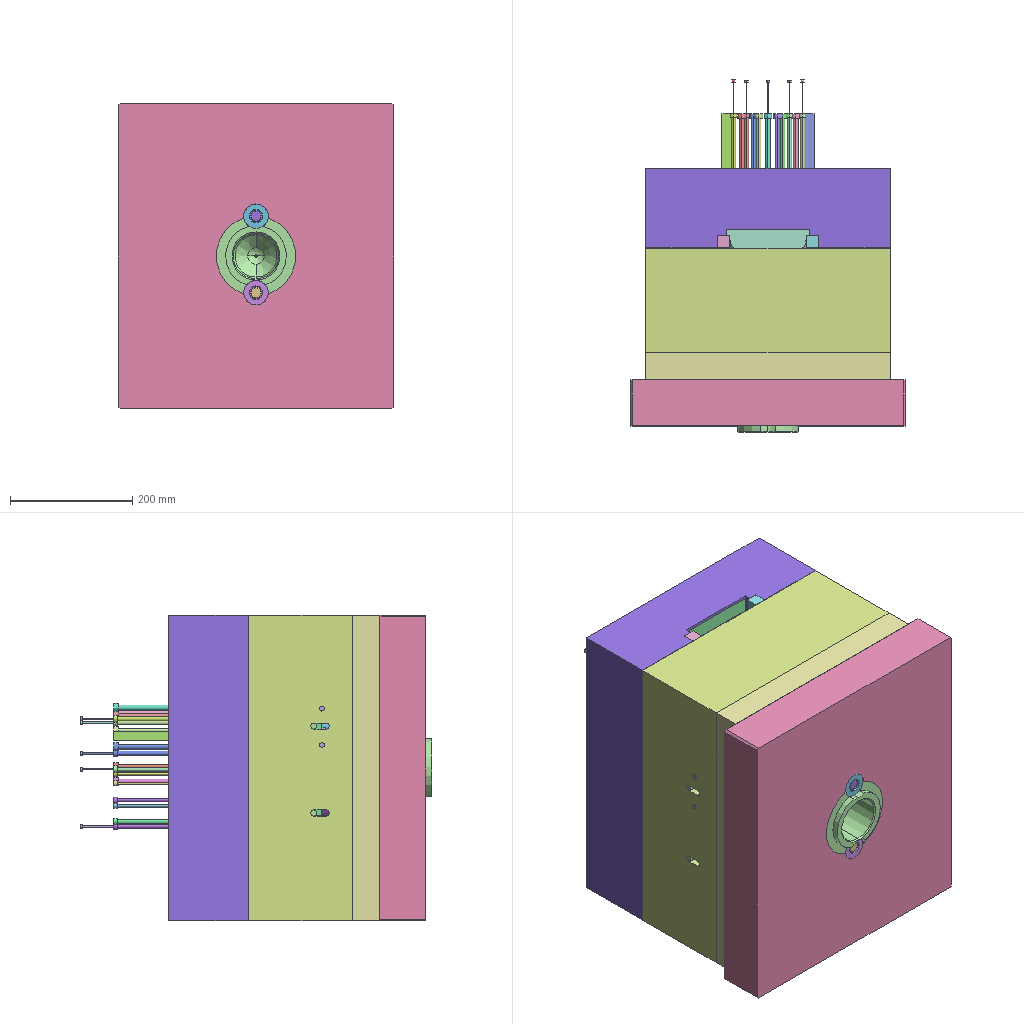Assembly | STEP file | 150 different items | 150 placed | box 450 x 576 x 500 mm
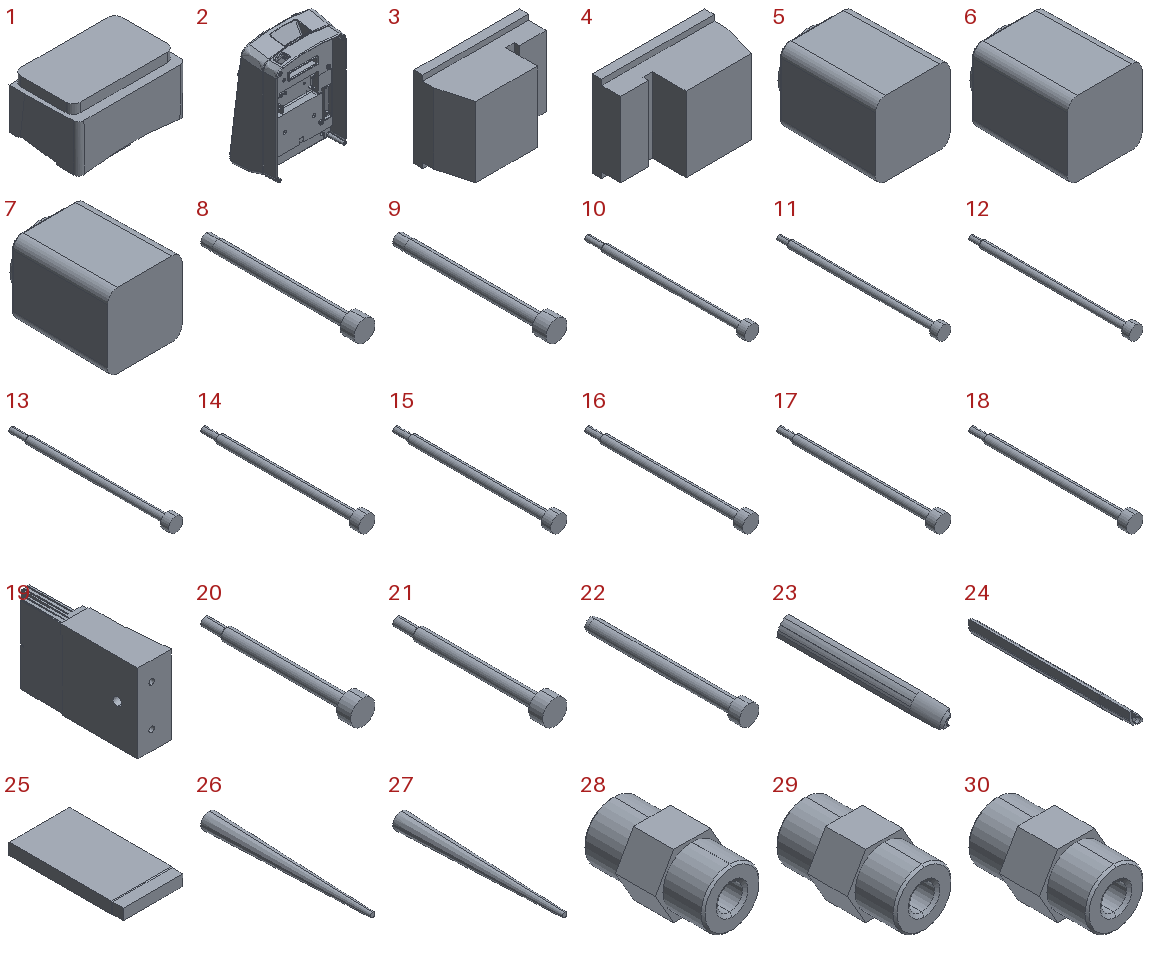Parts list (item | name | quantity | size | volume):
1 | (subassembly) | x1 | 119.805 x 74.045 x 84.64 mm | 483562 mm3
2 | 6022D002A | x1 | 145.669 x 91.672 x 216.186 mm | 218692 mm3
3 | (subassembly) | x1 | 60 x 30 x 46 mm | 59329 mm3
4 | (subassembly) | x1 | 60 x 30 x 46 mm | 59329 mm3
5 | (subassembly) | x1 | 11.23 x 15.729 x 11.23 mm | 1839 mm3
6 | (subassembly) | x1 | 11.23 x 15.729 x 11.23 mm | 1839 mm3
7 | (subassembly) | x1 | 11.23 x 15.729 x 11.23 mm | 1839 mm3
8 | (subassembly) | x1 | 9 x 68.14 x 9 mm | 1598 mm3
9 | (subassembly) | x1 | 9 x 68.14 x 9 mm | 1598 mm3
10 | (subassembly) | x1 | 7 x 79.697 x 7 mm | 843.527 mm3
11 | (subassembly) | x1 | 7 x 84.723 x 7 mm | 901.172 mm3
12 | (subassembly) | x1 | 7 x 84.723 x 7 mm | 901.172 mm3
13 | (subassembly) | x1 | 7 x 79.697 x 7 mm | 843.527 mm3
14 | (subassembly) | x1 | 7 x 69.447 x 7 mm | 750.263 mm3
15 | (subassembly) | x1 | 7 x 69.447 x 7 mm | 750.263 mm3
16 | (subassembly) | x1 | 7 x 69.447 x 7 mm | 750.263 mm3
17 | (subassembly) | x1 | 7 x 69.447 x 7 mm | 750.263 mm3
18 | (subassembly) | x1 | 7 x 69.447 x 7 mm | 750.263 mm3
19 | (subassembly) | x1 | 24.206 x 92.813 x 57.276 mm | 94075 mm3
20 | (subassembly) | x1 | 7 x 45.025 x 7 mm | 517.748 mm3
21 | (subassembly) | x1 | 7 x 45.025 x 7 mm | 517.748 mm3
22 | (subassembly) | x1 | 10 x 80.703 x 10 mm | 2941 mm3
23 | (subassembly) | x1 | 8.776 x 127.988 x 11.283 mm | 8417 mm3
24 | (subassembly) | x1 | 8.776 x 127.988 x 11.283 mm | 8418 mm3
25 | (subassembly) | x1 | 56.208 x 106.38 x 10.782 mm | 63955 mm3
26 | (subassembly) | x1 | 12.021 x 121.757 x 12.021 mm | 6349 mm3
27 | (subassembly) | x1 | 12.021 x 121.757 x 12.021 mm | 6349 mm3
28 | 6022D044 | x1 | 7.332 x 12 x 6.35 mm | 290.823 mm3
29 | 6022D044-1 | x1 | 7.332 x 12 x 6.35 mm | 290.823 mm3
30 | 6022D044-2 | x1 | 7.332 x 12 x 6.35 mm | 290.823 mm3
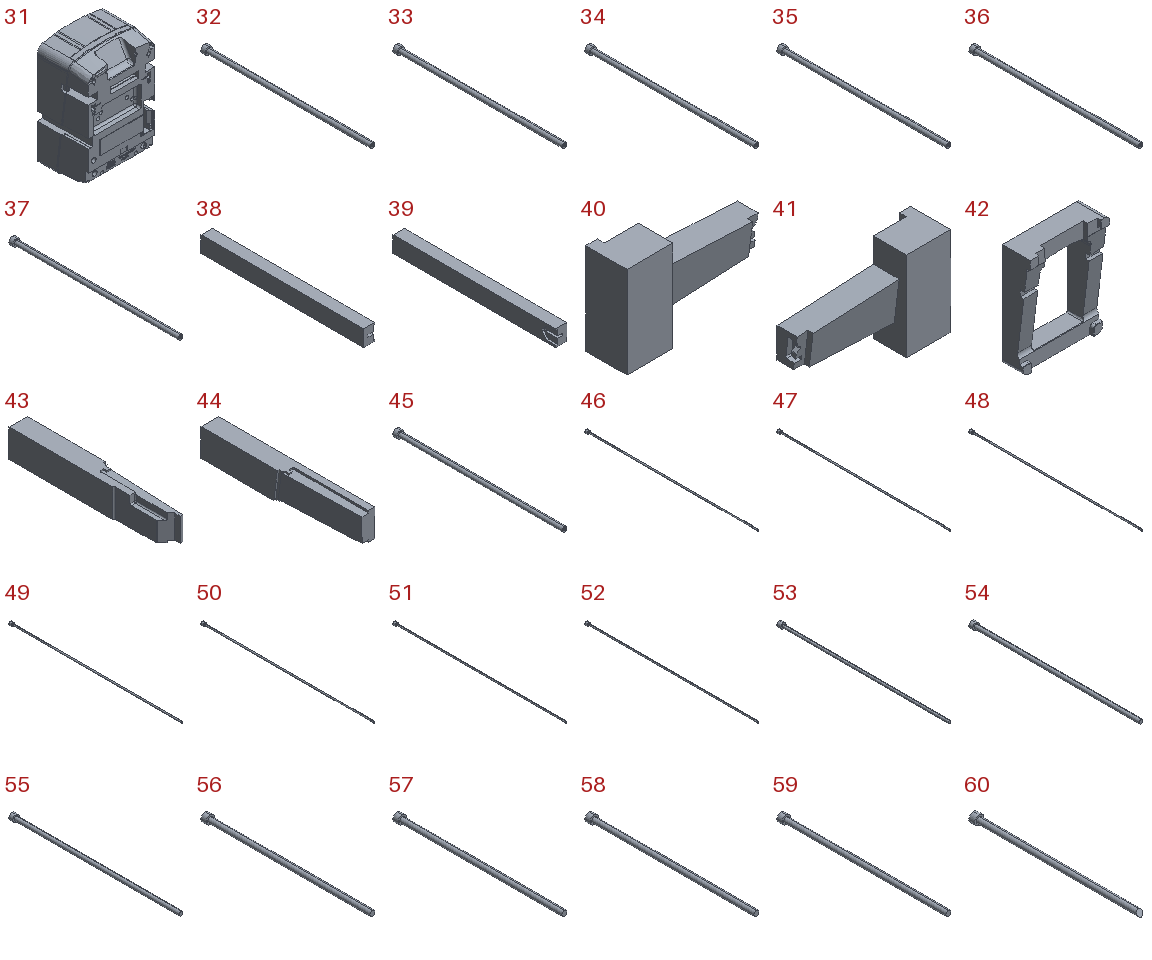31 | (subassembly) | x1 | 143.116 x 106.38 x 213.742 mm | 2647333 mm3
32 | (subassembly) | x1 | 11 x 244.986 x 11 mm | 8542 mm3
33 | (subassembly) | x1 | 11 x 244.986 x 11 mm | 8542 mm3
34 | (subassembly) | x1 | 11 x 244.986 x 11 mm | 8542 mm3
35 | (subassembly) | x1 | 11 x 244.986 x 11 mm | 8542 mm3
36 | (subassembly) | x1 | 11 x 243.265 x 11 mm | 8491 mm3
37 | (subassembly) | x1 | 11 x 254.534 x 11 mm | 8863 mm3
38 | (subassembly) | x1 | 7 x 102.36 x 10.193 mm | 7206 mm3
39 | (subassembly) | x1 | 7 x 102.36 x 10.193 mm | 7206 mm3
40 | (subassembly) | x1 | 63.268 x 18 x 40 mm | 19584 mm3
41 | (subassembly) | x1 | 63.268 x 18 x 40 mm | 19584 mm3
42 | (subassembly) | x1 | 220 x 78 x 290 mm | 1840139 mm3
43 | (subassembly) | x1 | 11.534 x 102.36 x 18.001 mm | 17054 mm3
44 | (subassembly) | x1 | 11.534 x 102.36 x 18.001 mm | 18637 mm3
45 | (subassembly) | x1 | 11 x 254.534 x 11 mm | 8863 mm3
46 | (subassembly) | x1 | 6 x 312.335 x 6 mm | 1622 mm3
47 | (subassembly) | x1 | 6 x 312.335 x 6 mm | 1622 mm3
48 | (subassembly) | x1 | 6 x 304.798 x 6 mm | 1589 mm3
49 | (subassembly) | x1 | 6 x 306.305 x 6 mm | 1597 mm3
50 | (subassembly) | x1 | 6 x 304.798 x 6 mm | 1589 mm3
51 | (subassembly) | x1 | 6 x 317.863 x 6 mm | 1651 mm3
52 | (subassembly) | x1 | 6 x 317.863 x 6 mm | 1651 mm3
53 | (subassembly) | x1 | 8 x 262.36 x 8 mm | 3523 mm3
54 | (subassembly) | x1 | 10 x 262.36 x 10 mm | 7720 mm3
55 | (subassembly) | x1 | 10 x 262.36 x 10 mm | 7720 mm3
56 | (subassembly) | x1 | 13 x 262.36 x 13 mm | 13847 mm3
57 | (subassembly) | x1 | 13 x 262.36 x 13 mm | 13847 mm3
58 | (subassembly) | x1 | 13 x 262.36 x 13 mm | 13847 mm3
59 | (subassembly) | x1 | 13 x 262.36 x 13 mm | 13847 mm3
60 | (subassembly) | x1 | 13 x 237.193 x 13 mm | 12467 mm3
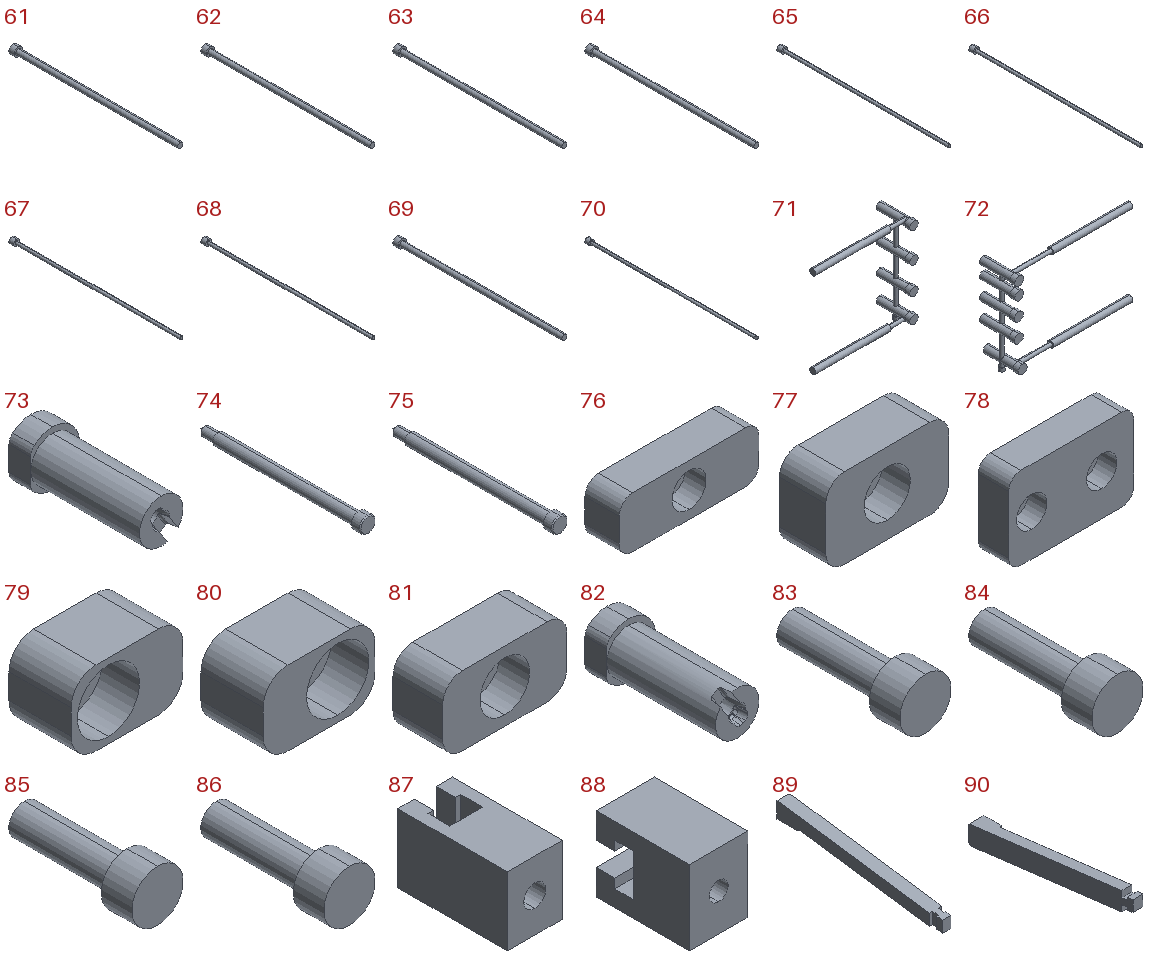61 | (subassembly) | x1 | 13 x 257.335 x 13 mm | 13595 mm3
62 | (subassembly) | x1 | 13 x 262.36 x 13 mm | 13847 mm3
63 | (subassembly) | x1 | 13 x 262.36 x 13 mm | 13847 mm3
64 | (subassembly) | x1 | 13 x 262.36 x 13 mm | 13847 mm3
65 | (subassembly) | x1 | 8 x 229.999 x 8 mm | 3116 mm3
66 | (subassembly) | x1 | 8 x 229.999 x 8 mm | 3116 mm3
67 | (subassembly) | x1 | 8 x 223.165 x 8 mm | 3031 mm3
68 | (subassembly) | x1 | 8 x 223.165 x 8 mm | 3031 mm3
69 | (subassembly) | x1 | 13 x 262.36 x 13 mm | 13847 mm3
70 | (subassembly) | x1 | 8 x 258.534 x 8 mm | 3450 mm3
71 | (subassembly) | x1 | 162 x 60 x 158.144 mm | 51671 mm3
72 | (subassembly) | x1 | 195 x 60 x 147.144 mm | 59737 mm3
73 | (subassembly) | x1 | 22.5 x 60 x 25 mm | 17728 mm3
74 | (subassembly) | x1 | 18 x 190 x 18 mm | 25064 mm3
75 | (subassembly) | x1 | 18 x 190 x 18 mm | 25064 mm3
76 | (subassembly) | x1 | 41 x 10 x 15 mm | 5428 mm3
77 | (subassembly) | x1 | 26.5 x 10 x 17.347 mm | 3875 mm3
78 | (subassembly) | x1 | 41 x 10 x 27 mm | 9764 mm3
79 | (subassembly) | x1 | 18 x 10 x 12 mm | 1438 mm3
80 | (subassembly) | x1 | 18 x 10 x 12 mm | 1438 mm3
81 | (subassembly) | x1 | 25.075 x 10 x 14 mm | 2789 mm3
82 | (subassembly) | x1 | 22.5 x 60 x 25 mm | 17728 mm3
83 | (subassembly) | x1 | 10 x 26 x 10 mm | 1037 mm3
84 | (subassembly) | x1 | 10 x 26 x 10 mm | 1037 mm3
85 | (subassembly) | x1 | 10 x 26 x 10 mm | 1037 mm3
86 | (subassembly) | x1 | 10 x 26 x 10 mm | 1037 mm3
87 | (subassembly) | x1 | 10 x 20 x 12.5 mm | 1868 mm3
88 | (subassembly) | x1 | 12.5 x 20 x 16 mm | 3149 mm3
89 | (subassembly) | x1 | 9 x 116.693 x 24.479 mm | 8518 mm3
90 | (subassembly) | x1 | 24.479 x 116.693 x 15 mm | 14289 mm3
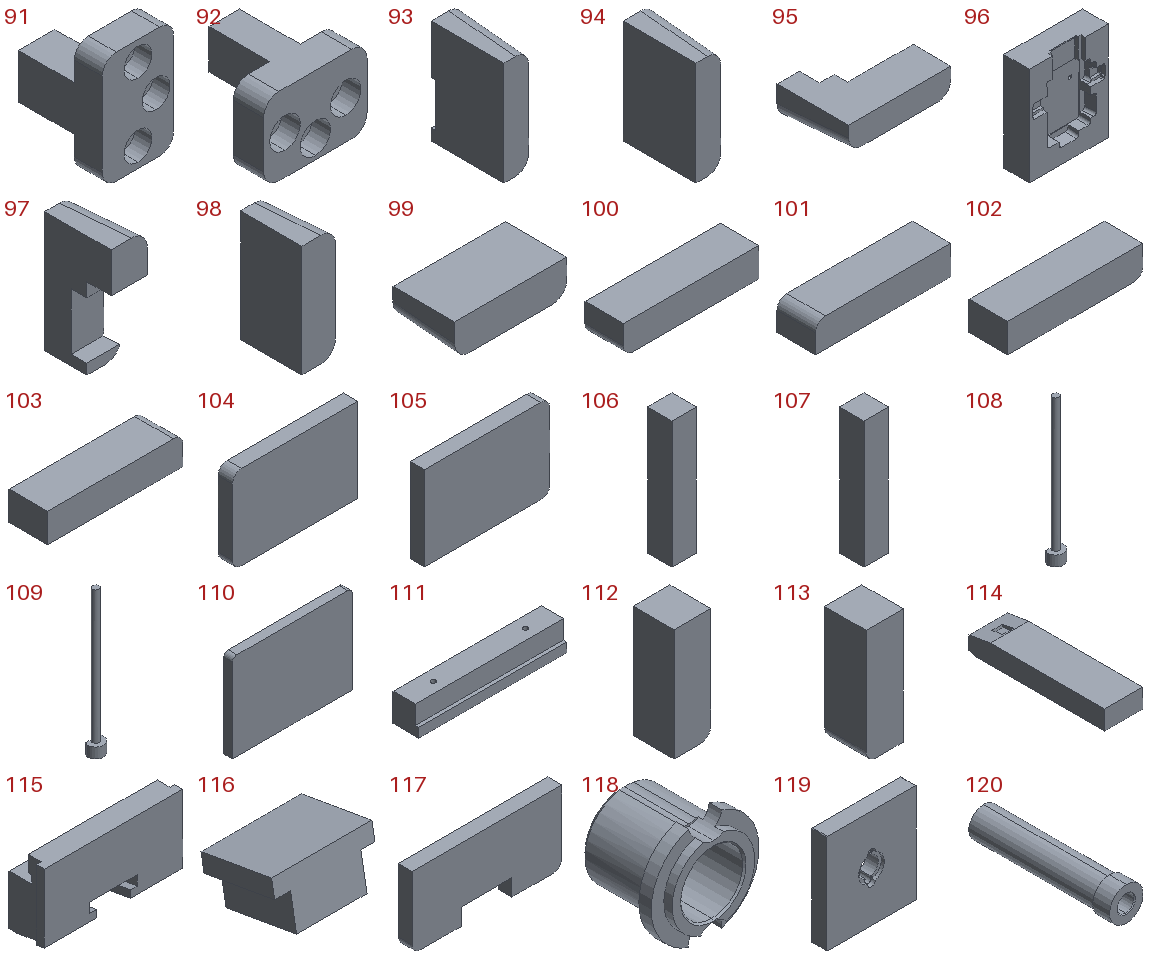91 | (subassembly) | x1 | 25.5 x 30 x 40 mm | 12392 mm3
92 | (subassembly) | x1 | 34 x 30 x 25.5 mm | 9302 mm3
93 | (subassembly) | x1 | 30 x 70 x 100 mm | 177836 mm3
94 | (subassembly) | x1 | 30 x 70 x 100 mm | 183468 mm3
95 | (subassembly) | x1 | 100 x 70 x 30 mm | 115912 mm3
96 | (subassembly) | x1 | 400 x 130 x 500 mm | 20837897 mm3
97 | (subassembly) | x1 | 30 x 55 x 100 mm | 92612 mm3
98 | (subassembly) | x1 | 30 x 55 x 100 mm | 147763 mm3
99 | (subassembly) | x1 | 100 x 55 x 30 mm | 147763 mm3
100 | (subassembly) | x1 | 70 x 20 x 15 mm | 20893 mm3
101 | (subassembly) | x1 | 70 x 20 x 15 mm | 20893 mm3
102 | (subassembly) | x1 | 70 x 20 x 15 mm | 20893 mm3
103 | (subassembly) | x1 | 70 x 20 x 15 mm | 20893 mm3
104 | (subassembly) | x1 | 70 x 8 x 47 mm | 26234 mm3
105 | (subassembly) | x1 | 70 x 8 x 47 mm | 26234 mm3
106 | (subassembly) | x1 | 20 x 20 x 105 mm | 42000 mm3
107 | (subassembly) | x1 | 20 x 20 x 105 mm | 42000 mm3
108 | (subassembly) | x1 | 6 x 4.256 x 55.458 mm | 340.576 mm3
109 | (subassembly) | x1 | 6 x 4.256 x 55.458 mm | 340.576 mm3
110 | (subassembly) | x1 | 136 x 10 x 100 mm | 135893 mm3
111 | (subassembly) | x1 | 80 x 14 x 15 mm | 14919 mm3
112 | (subassembly) | x1 | 18 x 20 x 55 mm | 19693 mm3
113 | (subassembly) | x1 | 18 x 20 x 56 mm | 20053 mm3
114 | (subassembly) | x1 | 70 x 250 x 35 mm | 599290 mm3
115 | (subassembly) | x1 | 86 x 25 x 46 mm | 68378 mm3
116 | (subassembly) | x1 | 28.5 x 22.681 x 18.312 mm | 6982 mm3
117 | (subassembly) | x1 | 87 x 8 x 41.949 mm | 26801 mm3
118 | (subassembly) | x1 | 130 x 132.5 x 123.637 mm | 522073 mm3
119 | (subassembly) | x1 | 450 x 75 x 500 mm | 16040639 mm3
120 | (subassembly) | x1 | 40 x 170 x 40 mm | 118148 mm3
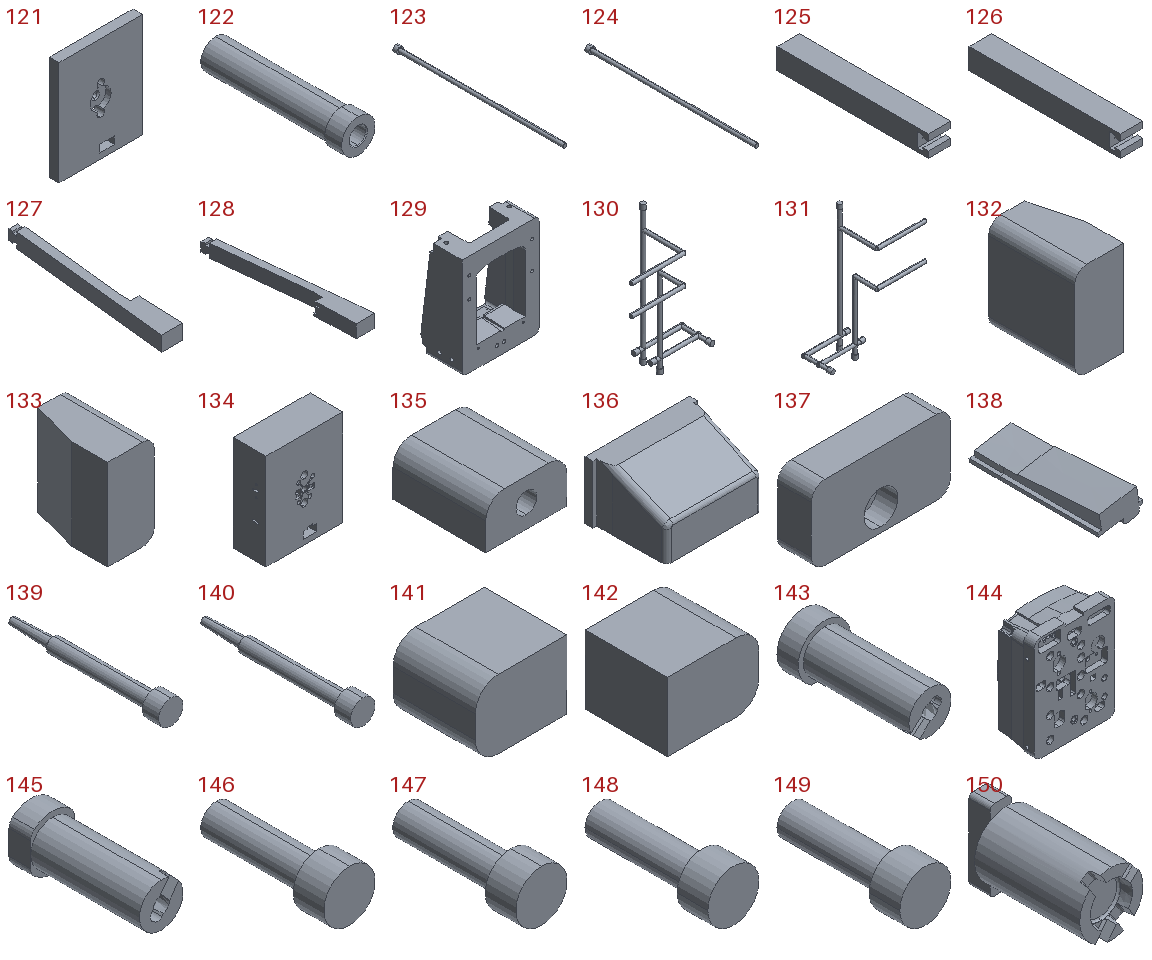121 | (subassembly) | x1 | 400 x 45 x 500 mm | 8595426 mm3
122 | (subassembly) | x1 | 40 x 170 x 40 mm | 118148 mm3
123 | (subassembly) | x1 | 10 x 257.335 x 10 mm | 7578 mm3
124 | (subassembly) | x1 | 10 x 257.335 x 10 mm | 7578 mm3
125 | (subassembly) | x1 | 16 x 108 x 15 mm | 24896 mm3
126 | (subassembly) | x1 | 16 x 108 x 15 mm | 24896 mm3
127 | (subassembly) | x1 | 24.981 x 162.36 x 14 mm | 24299 mm3
128 | (subassembly) | x1 | 24.981 x 162.36 x 14 mm | 24299 mm3
129 | (subassembly) | x1 | 220 x 118.069 x 290 mm | 3396178 mm3
130 | (subassembly) | x1 | 195 x 94 x 290 mm | 55392 mm3
131 | (subassembly) | x1 | 195 x 94 x 290 mm | 54387 mm3
132 | (subassembly) | x1 | 20 x 35.5 x 39 mm | 25224 mm3
133 | (subassembly) | x1 | 20 x 35.5 x 39 mm | 25224 mm3
134 | (subassembly) | x1 | 400 x 170 x 500 mm | 24400760 mm3
135 | (subassembly) | x1 | 35 x 40 x 20 mm | 23544 mm3
136 | (subassembly) | x1 | 135 x 99.045 x 75 mm | 726805 mm3
137 | (subassembly) | x1 | 41 x 10 x 22 mm | 8298 mm3
138 | (subassembly) | x1 | 21.719 x 62.11 x 12.971 mm | 7839 mm3
139 | (subassembly) | x1 | 6 x 38.743 x 6 mm | 385.655 mm3
140 | (subassembly) | x1 | 6 x 38.743 x 6 mm | 385.655 mm3
141 | (subassembly) | x1 | 20 x 18 x 15 mm | 5207 mm3
142 | (subassembly) | x1 | 20 x 18 x 15 mm | 5207 mm3
143 | (subassembly) | x1 | 25 x 60 x 23.412 mm | 17876 mm3
144 | (subassembly) | x1 | 150 x 88.701 x 195 mm | 1700421 mm3
145 | (subassembly) | x1 | 20 x 60 x 25 mm | 17460 mm3
146 | (subassembly) | x1 | 10 x 26 x 10 mm | 1037 mm3
147 | (subassembly) | x1 | 10 x 26 x 10 mm | 1037 mm3
148 | (subassembly) | x1 | 10 x 26 x 10 mm | 1037 mm3
149 | (subassembly) | x1 | 10 x 26 x 10 mm | 1037 mm3
150 | (subassembly) | x1 | 30 x 60 x 38 mm | 36750 mm3
Placements (level | parent | child | x y z in mm | rotation matrix by rows):
1 | subassembly 2 | subassembly 3 | -0.0 -0.0 -0.0 | 1 0 0 0 1 0 0 0 1
1 | subassembly 2 | 6022D002A | -0.0 -0.0 -0.0 | 1 0 0 0 1 0 0 0 1
1 | subassembly 2 | subassembly 4 | -0.0 -0.0 -0.0 | 1 0 0 0 1 0 0 0 1
1 | subassembly 2 | subassembly 5 | -0.0 -0.0 -0.0 | 1 0 0 0 1 0 0 0 1
1 | subassembly 2 | subassembly 6 | -0.0 -0.0 -0.0 | 1 0 0 0 1 0 0 0 1
1 | subassembly 2 | subassembly 7 | -0.0 -0.0 -0.0 | 1 0 0 0 1 0 0 0 1
1 | subassembly 2 | subassembly 8 | -0.0 -0.0 -0.0 | 1 0 0 0 1 0 0 0 1
1 | subassembly 2 | subassembly 9 | -0.0 -0.0 -0.0 | 1 0 0 0 1 0 0 0 1
1 | subassembly 2 | subassembly 10 | -0.0 -0.0 -0.0 | 1 0 0 0 1 0 0 0 1
1 | subassembly 2 | subassembly 11 | -0.0 -0.0 -0.0 | 1 0 0 0 1 0 0 0 1
1 | subassembly 2 | subassembly 12 | -0.0 -0.0 -0.0 | 1 0 0 0 1 0 0 0 1
1 | subassembly 2 | subassembly 13 | -0.0 -0.0 -0.0 | 1 0 0 0 1 0 0 0 1
1 | subassembly 2 | subassembly 14 | -0.0 -0.0 -0.0 | 1 0 0 0 1 0 0 0 1
1 | subassembly 2 | subassembly 15 | -0.0 -0.0 -0.0 | 1 0 0 0 1 0 0 0 1
1 | subassembly 2 | subassembly 16 | -0.0 -0.0 -0.0 | 1 0 0 0 1 0 0 0 1
1 | subassembly 2 | subassembly 17 | -0.0 -0.0 -0.0 | 1 0 0 0 1 0 0 0 1
1 | subassembly 2 | subassembly 18 | -0.0 -0.0 -0.0 | 1 0 0 0 1 0 0 0 1
1 | subassembly 2 | subassembly 19 | -0.0 -0.0 -0.0 | 1 0 0 0 1 0 0 0 1
1 | subassembly 2 | subassembly 20 | -0.0 -0.0 -0.0 | 1 0 0 0 1 0 0 0 1
1 | subassembly 2 | subassembly 21 | -0.0 -0.0 -0.0 | 1 0 0 0 1 0 0 0 1
1 | subassembly 2 | subassembly 22 | -0.0 -0.0 -0.0 | 1 0 0 0 1 0 0 0 1
1 | subassembly 2 | subassembly 23 | -0.0 -0.0 -0.0 | 1 0 0 0 1 0 0 0 1
1 | subassembly 2 | subassembly 24 | -0.0 -0.0 -0.0 | 1 0 0 0 1 0 0 0 1
1 | subassembly 2 | subassembly 25 | -0.0 -0.0 -0.0 | 1 0 0 0 1 0 0 0 1
1 | subassembly 2 | subassembly 26 | -0.0 -0.0 -0.0 | 1 0 0 0 1 0 0 0 1
1 | subassembly 2 | subassembly 27 | -0.0 -0.0 -0.0 | 1 0 0 0 1 0 0 0 1
1 | subassembly 2 | subassembly 28 | -0.0 -0.0 -0.0 | 1 0 0 0 1 0 0 0 1
1 | subassembly 2 | 6022D044 | -0.0 -0.0 -0.0 | 1 0 0 0 1 0 0 0 1
1 | subassembly 2 | 6022D044-1 | -0.0 -0.0 -0.0 | 1 0 0 0 1 0 0 0 1
1 | subassembly 2 | 6022D044-2 | -0.0 -0.0 -0.0 | 1 0 0 0 1 0 0 0 1
1 | subassembly 2 | subassembly 29 | -0.0 -0.0 -0.0 | 1 0 0 0 1 0 0 0 1
1 | subassembly 2 | subassembly 30 | -0.0 -0.0 -0.0 | 1 0 0 0 1 0 0 0 1
1 | subassembly 2 | subassembly 31 | -0.0 -0.0 -0.0 | 1 0 0 0 1 0 0 0 1
1 | subassembly 2 | subassembly 32 | -0.0 -0.0 -0.0 | 1 0 0 0 1 0 0 0 1
1 | subassembly 2 | subassembly 33 | -0.0 -0.0 -0.0 | 1 0 0 0 1 0 0 0 1
1 | subassembly 2 | subassembly 34 | -0.0 -0.0 -0.0 | 1 0 0 0 1 0 0 0 1
1 | subassembly 2 | subassembly 35 | -0.0 -0.0 -0.0 | 1 0 0 0 1 0 0 0 1
1 | subassembly 2 | subassembly 36 | -0.0 -0.0 -0.0 | 1 0 0 0 1 0 0 0 1
1 | subassembly 2 | subassembly 37 | -0.0 -0.0 -0.0 | 1 0 0 0 1 0 0 0 1
1 | subassembly 2 | subassembly 38 | -0.0 -0.0 -0.0 | 1 0 0 0 1 0 0 0 1
1 | subassembly 2 | subassembly 39 | -0.0 -0.0 -0.0 | 1 0 0 0 1 0 0 0 1
1 | subassembly 2 | subassembly 40 | -0.0 -0.0 -0.0 | 1 0 0 0 1 0 0 0 1
1 | subassembly 2 | subassembly 41 | -0.0 -0.0 -0.0 | 1 0 0 0 1 0 0 0 1
1 | subassembly 2 | subassembly 42 | -0.0 -0.0 -0.0 | 1 0 0 0 1 0 0 0 1
1 | subassembly 2 | subassembly 43 | -0.0 -0.0 -0.0 | 1 0 0 0 1 0 0 0 1
1 | subassembly 2 | subassembly 44 | -0.0 -0.0 -0.0 | 1 0 0 0 1 0 0 0 1
1 | subassembly 2 | subassembly 45 | -0.0 -0.0 -0.0 | 1 0 0 0 1 0 0 0 1
1 | subassembly 2 | subassembly 46 | -0.0 -0.0 -0.0 | 1 0 0 0 1 0 0 0 1
1 | subassembly 2 | subassembly 47 | -0.0 -0.0 -0.0 | 1 0 0 0 1 0 0 0 1
1 | subassembly 2 | subassembly 48 | -0.0 -0.0 -0.0 | 1 0 0 0 1 0 0 0 1
1 | subassembly 2 | subassembly 49 | -0.0 -0.0 -0.0 | 1 0 0 0 1 0 0 0 1
1 | subassembly 2 | subassembly 50 | -0.0 -0.0 -0.0 | 1 0 0 0 1 0 0 0 1
1 | subassembly 2 | subassembly 51 | -0.0 -0.0 -0.0 | 1 0 0 0 1 0 0 0 1
1 | subassembly 2 | subassembly 52 | -0.0 -0.0 -0.0 | 1 0 0 0 1 0 0 0 1
1 | subassembly 2 | subassembly 53 | -0.0 -0.0 -0.0 | 1 0 0 0 1 0 0 0 1
1 | subassembly 2 | subassembly 54 | -0.0 -0.0 -0.0 | 1 0 0 0 1 0 0 0 1
1 | subassembly 2 | subassembly 55 | -0.0 -0.0 -0.0 | 1 0 0 0 1 0 0 0 1
1 | subassembly 2 | subassembly 56 | -0.0 -0.0 -0.0 | 1 0 0 0 1 0 0 0 1
1 | subassembly 2 | subassembly 57 | -0.0 -0.0 -0.0 | 1 0 0 0 1 0 0 0 1
1 | subassembly 2 | subassembly 58 | -0.0 -0.0 -0.0 | 1 0 0 0 1 0 0 0 1
1 | subassembly 2 | subassembly 59 | -0.0 -0.0 -0.0 | 1 0 0 0 1 0 0 0 1
1 | subassembly 2 | subassembly 60 | -0.0 -0.0 -0.0 | 1 0 0 0 1 0 0 0 1
1 | subassembly 2 | subassembly 61 | -0.0 -0.0 -0.0 | 1 0 0 0 1 0 0 0 1
1 | subassembly 2 | subassembly 62 | -0.0 -0.0 -0.0 | 1 0 0 0 1 0 0 0 1
1 | subassembly 2 | subassembly 63 | -0.0 -0.0 -0.0 | 1 0 0 0 1 0 0 0 1
1 | subassembly 2 | subassembly 64 | -0.0 -0.0 -0.0 | 1 0 0 0 1 0 0 0 1
1 | subassembly 2 | subassembly 65 | -0.0 -0.0 -0.0 | 1 0 0 0 1 0 0 0 1
1 | subassembly 2 | subassembly 66 | -0.0 -0.0 -0.0 | 1 0 0 0 1 0 0 0 1
1 | subassembly 2 | subassembly 67 | -0.0 -0.0 -0.0 | 1 0 0 0 1 0 0 0 1
1 | subassembly 2 | subassembly 68 | -0.0 -0.0 -0.0 | 1 0 0 0 1 0 0 0 1
1 | subassembly 2 | subassembly 69 | -0.0 -0.0 -0.0 | 1 0 0 0 1 0 0 0 1
1 | subassembly 2 | subassembly 70 | -0.0 -0.0 -0.0 | 1 0 0 0 1 0 0 0 1
1 | subassembly 2 | subassembly 71 | -0.0 -0.0 -0.0 | 1 0 0 0 1 0 0 0 1
1 | subassembly 2 | subassembly 72 | -0.0 -0.0 -0.0 | 1 0 0 0 1 0 0 0 1
1 | subassembly 2 | subassembly 73 | -0.0 -0.0 -0.0 | 1 0 0 0 1 0 0 0 1
1 | subassembly 2 | subassembly 74 | -0.0 -0.0 -0.0 | 1 0 0 0 1 0 0 0 1
1 | subassembly 2 | subassembly 75 | -0.0 -0.0 -0.0 | 1 0 0 0 1 0 0 0 1
1 | subassembly 2 | subassembly 76 | -0.0 -0.0 -0.0 | 1 0 0 0 1 0 0 0 1
1 | subassembly 2 | subassembly 77 | -0.0 -0.0 -0.0 | 1 0 0 0 1 0 0 0 1
1 | subassembly 2 | subassembly 78 | -0.0 -0.0 -0.0 | 1 0 0 0 1 0 0 0 1
1 | subassembly 2 | subassembly 79 | -0.0 -0.0 -0.0 | 1 0 0 0 1 0 0 0 1
1 | subassembly 2 | subassembly 80 | -0.0 -0.0 -0.0 | 1 0 0 0 1 0 0 0 1
1 | subassembly 2 | subassembly 81 | -0.0 -0.0 -0.0 | 1 0 0 0 1 0 0 0 1
1 | subassembly 2 | subassembly 82 | -0.0 -0.0 -0.0 | 1 0 0 0 1 0 0 0 1
1 | subassembly 2 | subassembly 83 | -0.0 -0.0 -0.0 | 1 0 0 0 1 0 0 0 1
1 | subassembly 2 | subassembly 84 | -0.0 -0.0 -0.0 | 1 0 0 0 1 0 0 0 1
1 | subassembly 2 | subassembly 85 | -0.0 -0.0 -0.0 | 1 0 0 0 1 0 0 0 1
1 | subassembly 2 | subassembly 86 | -0.0 -0.0 -0.0 | 1 0 0 0 1 0 0 0 1
1 | subassembly 2 | subassembly 87 | -0.0 -0.0 -0.0 | 1 0 0 0 1 0 0 0 1
1 | subassembly 2 | subassembly 88 | -0.0 -0.0 -0.0 | 1 0 0 0 1 0 0 0 1
1 | subassembly 2 | subassembly 89 | -0.0 -0.0 -0.0 | 1 0 0 0 1 0 0 0 1
1 | subassembly 2 | subassembly 90 | -0.0 -0.0 -0.0 | 1 0 0 0 1 0 0 0 1
1 | subassembly 2 | subassembly 91 | -0.0 -0.0 -0.0 | 1 0 0 0 1 0 0 0 1
1 | subassembly 2 | subassembly 92 | -0.0 -0.0 -0.0 | 1 0 0 0 1 0 0 0 1
1 | subassembly 2 | subassembly 93 | -0.0 -0.0 -0.0 | 1 0 0 0 1 0 0 0 1
1 | subassembly 2 | subassembly 94 | -0.0 -0.0 -0.0 | 1 0 0 0 1 0 0 0 1
1 | subassembly 2 | subassembly 95 | -0.0 -0.0 -0.0 | 1 0 0 0 1 0 0 0 1
1 | subassembly 2 | subassembly 96 | -0.0 -0.0 -0.0 | 1 0 0 0 1 0 0 0 1
1 | subassembly 2 | subassembly 97 | -0.0 -0.0 -0.0 | 1 0 0 0 1 0 0 0 1
1 | subassembly 2 | subassembly 98 | -0.0 -0.0 -0.0 | 1 0 0 0 1 0 0 0 1
1 | subassembly 2 | subassembly 99 | -0.0 -0.0 -0.0 | 1 0 0 0 1 0 0 0 1
1 | subassembly 2 | subassembly 100 | -0.0 -0.0 -0.0 | 1 0 0 0 1 0 0 0 1
1 | subassembly 2 | subassembly 101 | -0.0 -0.0 -0.0 | 1 0 0 0 1 0 0 0 1
1 | subassembly 2 | subassembly 102 | -0.0 -0.0 -0.0 | 1 0 0 0 1 0 0 0 1
1 | subassembly 2 | subassembly 103 | -0.0 -0.0 -0.0 | 1 0 0 0 1 0 0 0 1
1 | subassembly 2 | subassembly 104 | -0.0 -0.0 -0.0 | 1 0 0 0 1 0 0 0 1
1 | subassembly 2 | subassembly 105 | -0.0 -0.0 -0.0 | 1 0 0 0 1 0 0 0 1
1 | subassembly 2 | subassembly 106 | -0.0 -0.0 -0.0 | 1 0 0 0 1 0 0 0 1
1 | subassembly 2 | subassembly 107 | -0.0 -0.0 -0.0 | 1 0 0 0 1 0 0 0 1
1 | subassembly 2 | subassembly 108 | -0.0 -0.0 -0.0 | 1 0 0 0 1 0 0 0 1
1 | subassembly 2 | subassembly 109 | -0.0 -0.0 -0.0 | 1 0 0 0 1 0 0 0 1
1 | subassembly 2 | subassembly 110 | -0.0 -0.0 -0.0 | 1 0 0 0 1 0 0 0 1
1 | subassembly 2 | subassembly 111 | -0.0 -0.0 -0.0 | 1 0 0 0 1 0 0 0 1
1 | subassembly 2 | subassembly 112 | -0.0 -0.0 -0.0 | 1 0 0 0 1 0 0 0 1
1 | subassembly 2 | subassembly 113 | -0.0 -0.0 -0.0 | 1 0 0 0 1 0 0 0 1
1 | subassembly 2 | subassembly 114 | -0.0 -0.0 -0.0 | 1 0 0 0 1 0 0 0 1
1 | subassembly 2 | subassembly 115 | -0.0 -0.0 -0.0 | 1 0 0 0 1 0 0 0 1
1 | subassembly 2 | subassembly 116 | -0.0 -0.0 -0.0 | 1 0 0 0 1 0 0 0 1
1 | subassembly 2 | subassembly 117 | -0.0 -0.0 -0.0 | 1 0 0 0 1 0 0 0 1
1 | subassembly 2 | subassembly 118 | -0.0 -0.0 -0.0 | 1 0 0 0 1 0 0 0 1
1 | subassembly 2 | subassembly 119 | -0.0 -0.0 -0.0 | 1 0 0 0 1 0 0 0 1
1 | subassembly 2 | subassembly 120 | -0.0 -0.0 -0.0 | 1 0 0 0 1 0 0 0 1
1 | subassembly 2 | subassembly 121 | -0.0 -0.0 -0.0 | 1 0 0 0 1 0 0 0 1
1 | subassembly 2 | subassembly 122 | -0.0 -0.0 -0.0 | 1 0 0 0 1 0 0 0 1
1 | subassembly 2 | subassembly 123 | -0.0 -0.0 -0.0 | 1 0 0 0 1 0 0 0 1
1 | subassembly 2 | subassembly 124 | -0.0 -0.0 -0.0 | 1 0 0 0 1 0 0 0 1
1 | subassembly 2 | subassembly 125 | -0.0 -0.0 -0.0 | 1 0 0 0 1 0 0 0 1
1 | subassembly 2 | subassembly 126 | -0.0 -0.0 -0.0 | 1 0 0 0 1 0 0 0 1
1 | subassembly 2 | subassembly 127 | -0.0 -0.0 -0.0 | 1 0 0 0 1 0 0 0 1
1 | subassembly 2 | subassembly 128 | -0.0 -0.0 -0.0 | 1 0 0 0 1 0 0 0 1
1 | subassembly 2 | subassembly 129 | -0.0 -0.0 -0.0 | 1 0 0 0 1 0 0 0 1
1 | subassembly 2 | subassembly 130 | -0.0 -0.0 -0.0 | 1 0 0 0 1 0 0 0 1
1 | subassembly 2 | subassembly 131 | -0.0 -0.0 -0.0 | 1 0 0 0 1 0 0 0 1
1 | subassembly 2 | subassembly 132 | -0.0 -0.0 -0.0 | 1 0 0 0 1 0 0 0 1
1 | subassembly 2 | subassembly 133 | -0.0 -0.0 -0.0 | 1 0 0 0 1 0 0 0 1
1 | subassembly 2 | subassembly 134 | -0.0 -0.0 -0.0 | 1 0 0 0 1 0 0 0 1
1 | subassembly 2 | subassembly 135 | -0.0 -0.0 -0.0 | 1 0 0 0 1 0 0 0 1
1 | subassembly 2 | subassembly 136 | -0.0 -0.0 -0.0 | 1 0 0 0 1 0 0 0 1
1 | subassembly 2 | subassembly 137 | -0.0 -0.0 -0.0 | 1 0 0 0 1 0 0 0 1
1 | subassembly 2 | subassembly 138 | -0.0 -0.0 -0.0 | 1 0 0 0 1 0 0 0 1
1 | subassembly 2 | subassembly 139 | -0.0 -0.0 -0.0 | 1 0 0 0 1 0 0 0 1
1 | subassembly 2 | subassembly 140 | -0.0 -0.0 -0.0 | 1 0 0 0 1 0 0 0 1
1 | subassembly 2 | subassembly 141 | -0.0 -0.0 -0.0 | 1 0 0 0 1 0 0 0 1
1 | subassembly 2 | subassembly 142 | -0.0 -0.0 -0.0 | 1 0 0 0 1 0 0 0 1
1 | subassembly 2 | subassembly 143 | -0.0 -0.0 -0.0 | 1 0 0 0 1 0 0 0 1
1 | subassembly 2 | subassembly 144 | -0.0 -0.0 -0.0 | 1 0 0 0 1 0 0 0 1
1 | subassembly 2 | subassembly 145 | -0.0 -0.0 -0.0 | 1 0 0 0 1 0 0 0 1
1 | subassembly 2 | subassembly 146 | -0.0 -0.0 -0.0 | 1 0 0 0 1 0 0 0 1
1 | subassembly 2 | subassembly 147 | -0.0 -0.0 -0.0 | 1 0 0 0 1 0 0 0 1
1 | subassembly 2 | subassembly 148 | -0.0 -0.0 -0.0 | 1 0 0 0 1 0 0 0 1